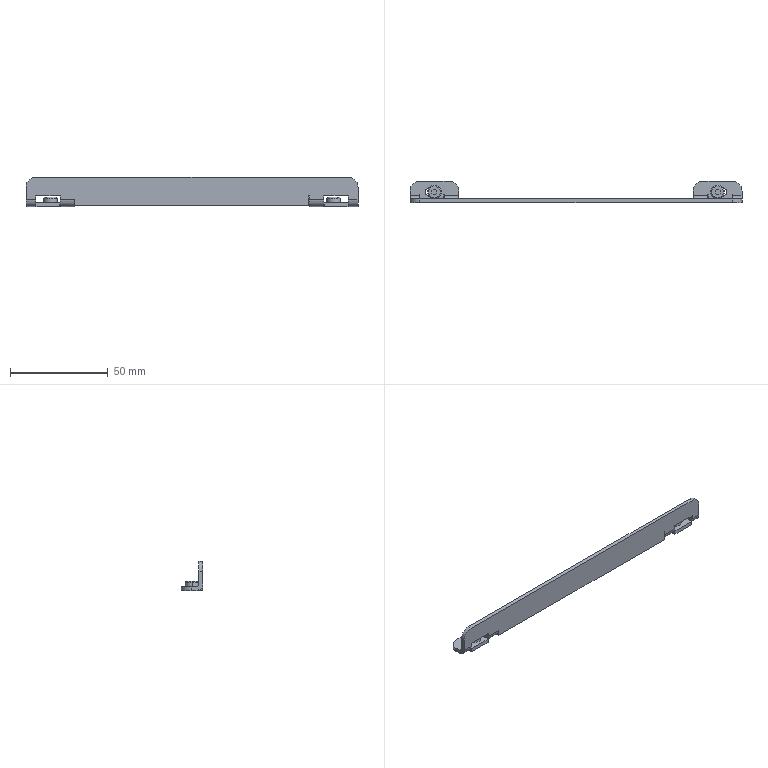Part | STEP file | _Schaltwinkel l170-SBG - PAS42 B | 1 solid | 83 faces | box 170 x 11 x 15 mm | volume 5664 mm3 | plane 55 | cylinder 24 | cone 4 | commonest cylinder face diameters 7 x8 4.5 x6 10 x6 3 x4